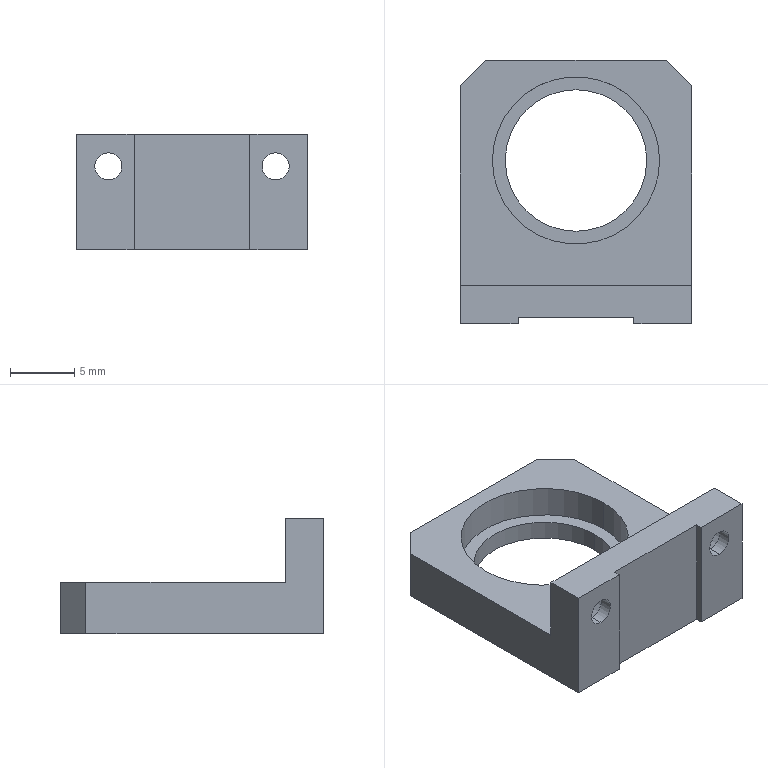Part | SolidWorks | features MoveFace 4, ICE 2, BaseBody 1, Chamfer 1, DelFace 1, HoleWzd 1 | 1 solid | 29 faces | box 18 x 20.5 x 9 mm | volume 1150 mm3 | plane 17 | cylinder 12 | commonest cylinder face diameters 2.1 x4 4.3 x4 11 x2 13 x2
STEP:
#1=CARTESIAN_POINT('',(6.,1.,7.6));
#2=VERTEX_POINT('',#1);
#3=CARTESIAN_POINT('',(6.,1.,11.9));
#4=VERTEX_POINT('',#3);
#5=CARTESIAN_POINT('',(6.,1.,9.75));
#6=DIRECTION('',(0.,1.,0.));
#7=DIRECTION('',(0.,0.,1.));
#8=AXIS2_PLACEMENT_3D('',#5,#6,#7);
#9=CIRCLE('',#8,2.15);
#10=EDGE_CURVE('',#2,#4,#9,.T.);
#11=ORIENTED_EDGE('',*,*,#10,.F.);
#12=CARTESIAN_POINT('',(6.,3.,7.6));
#13=VERTEX_POINT('',#12);
#14=CARTESIAN_POINT('',(6.,3.,7.6));
#15=DIRECTION('',(0.,1.,0.));
#16=VECTOR('',#15,1000.);
#17=LINE('',#14,#16);
#18=EDGE_CURVE('',#2,#13,#17,.T.);
#19=ORIENTED_EDGE('',*,*,#18,.T.);
#20=CARTESIAN_POINT('',(6.,3.,11.9));
#21=VERTEX_POINT('',#20);
#22=CARTESIAN_POINT('',(6.,3.,9.75));
#23=DIRECTION('',(0.,1.,0.));
#24=DIRECTION('',(0.,0.,1.));
#25=AXIS2_PLACEMENT_3D('',#22,#23,#24);
#26=CIRCLE('',#25,2.15);
#27=EDGE_CURVE('',#13,#21,#26,.T.);
#28=ORIENTED_EDGE('',*,*,#27,.T.);
#29=CARTESIAN_POINT('',(6.,3.,11.9));
#30=DIRECTION('',(0.,1.,0.));
#31=VECTOR('',#30,1000.);
#32=LINE('',#29,#31);
#33=EDGE_CURVE('',#4,#21,#32,.T.);
#34=ORIENTED_EDGE('',*,*,#33,.F.);
#35=EDGE_LOOP('',(#11,#19,#28,#34));
#36=FACE_OUTER_BOUND('',#35,.T.);
#37=CARTESIAN_POINT('',(6.,3.,9.75));
#38=DIRECTION('',(0.,1.,0.));
#39=DIRECTION('',(0.,0.,1.));
#40=AXIS2_PLACEMENT_3D('',#37,#38,#39);
#41=CYLINDRICAL_SURFACE('',#40,2.15);
#42=ADVANCED_FACE('',(#36),#41,.F.);
#43=CARTESIAN_POINT('',(6.,0.,10.8));
#44=VERTEX_POINT('',#43);
#45=CARTESIAN_POINT('',(6.,0.,8.7));
#46=VERTEX_POINT('',#45);
#47=CARTESIAN_POINT('',(6.,0.,9.75));
#48=DIRECTION('',(0.,-1.,0.));
#49=DIRECTION('',(0.,0.,-1.));
#50=AXIS2_PLACEMENT_3D('',#47,#48,#49);
#51=CIRCLE('',#50,1.05);
#52=EDGE_CURVE('',#44,#46,#51,.T.);
#53=ORIENTED_EDGE('',*,*,#52,.T.);
#54=CARTESIAN_POINT('',(6.,1.,8.7));
#55=VERTEX_POINT('',#54);
#56=CARTESIAN_POINT('',(6.,3.,8.7));
#57=DIRECTION('',(0.,1.,0.));
#58=VECTOR('',#57,1000.);
#59=LINE('',#56,#58);
#60=EDGE_CURVE('',#46,#55,#59,.T.);
#61=ORIENTED_EDGE('',*,*,#60,.T.);
#62=CARTESIAN_POINT('',(6.,1.,10.8));
#63=VERTEX_POINT('',#62);
#64=CARTESIAN_POINT('',(6.,1.,9.75));
#65=DIRECTION('',(0.,1.,0.));
#66=DIRECTION('',(0.,0.,1.));
#67=AXIS2_PLACEMENT_3D('',#64,#65,#66);
#68=CIRCLE('',#67,1.05);
#69=EDGE_CURVE('',#55,#63,#68,.T.);
#70=ORIENTED_EDGE('',*,*,#69,.T.);
#71=CARTESIAN_POINT('',(6.,3.,10.8));
#72=DIRECTION('',(0.,1.,0.));
#73=VECTOR('',#72,1000.);
#74=LINE('',#71,#73);
#75=EDGE_CURVE('',#44,#63,#74,.T.);
#76=ORIENTED_EDGE('',*,*,#75,.F.);
#77=EDGE_LOOP('',(#53,#61,#70,#76));
#78=FACE_OUTER_BOUND('',#77,.T.);
#79=CARTESIAN_POINT('',(6.,3.,9.75));
#80=DIRECTION('',(0.,1.,0.));
#81=DIRECTION('',(0.,0.,1.));
#82=AXIS2_PLACEMENT_3D('',#79,#80,#81);
#83=CYLINDRICAL_SURFACE('',#82,1.05);
#84=ADVANCED_FACE('',(#78),#83,.F.);
#85=CARTESIAN_POINT('',(19.,1.,7.6));
#86=VERTEX_POINT('',#85);
#87=CARTESIAN_POINT('',(19.,1.,11.9));
#88=VERTEX_POINT('',#87);
#89=CARTESIAN_POINT('',(19.,1.,9.75));
#90=DIRECTION('',(0.,1.,0.));
#91=DIRECTION('',(0.,0.,1.));
#92=AXIS2_PLACEMENT_3D('',#89,#90,#91);
#93=CIRCLE('',#92,2.15);
#94=EDGE_CURVE('',#86,#88,#93,.T.);
#95=ORIENTED_EDGE('',*,*,#94,.F.);
#96=CARTESIAN_POINT('',(19.,3.,7.6));
#97=VERTEX_POINT('',#96);
#98=CARTESIAN_POINT('',(19.,3.,7.6));
#99=DIRECTION('',(0.,1.,0.));
#100=VECTOR('',#99,1000.);
#101=LINE('',#98,#100);
#102=EDGE_CURVE('',#86,#97,#101,.T.);
#103=ORIENTED_EDGE('',*,*,#102,.T.);
#104=CARTESIAN_POINT('',(19.,3.,11.9));
#105=VERTEX_POINT('',#104);
#106=CARTESIAN_POINT('',(19.,3.,9.75));
#107=DIRECTION('',(0.,1.,0.));
#108=DIRECTION('',(0.,0.,1.));
#109=AXIS2_PLACEMENT_3D('',#106,#107,#108);
#110=CIRCLE('',#109,2.15);
#111=EDGE_CURVE('',#97,#105,#110,.T.);
#112=ORIENTED_EDGE('',*,*,#111,.T.);
#113=CARTESIAN_POINT('',(19.,3.,11.9));
#114=DIRECTION('',(0.,1.,0.));
#115=VECTOR('',#114,1000.);
#116=LINE('',#113,#115);
#117=EDGE_CURVE('',#88,#105,#116,.T.);
#118=ORIENTED_EDGE('',*,*,#117,.F.);
#119=EDGE_LOOP('',(#95,#103,#112,#118));
#120=FACE_OUTER_BOUND('',#119,.T.);
#121=CARTESIAN_POINT('',(19.,3.,9.75));
#122=DIRECTION('',(0.,1.,0.));
#123=DIRECTION('',(0.,0.,1.));
#124=AXIS2_PLACEMENT_3D('',#121,#122,#123);
#125=CYLINDRICAL_SURFACE('',#124,2.15);
#126=ADVANCED_FACE('',(#120),#125,.F.);
#127=CARTESIAN_POINT('',(19.,0.,10.8));
#128=VERTEX_POINT('',#127);
#129=CARTESIAN_POINT('',(19.,0.,8.7));
#130=VERTEX_POINT('',#129);
#131=CARTESIAN_POINT('',(19.,0.,9.75));
#132=DIRECTION('',(0.,-1.,0.));
#133=DIRECTION('',(0.,0.,-1.));
#134=AXIS2_PLACEMENT_3D('',#131,#132,#133);
#135=CIRCLE('',#134,1.05);
#136=EDGE_CURVE('',#128,#130,#135,.T.);
#137=ORIENTED_EDGE('',*,*,#136,.T.);
#138=CARTESIAN_POINT('',(19.,1.,8.7));
#139=VERTEX_POINT('',#138);
#140=CARTESIAN_POINT('',(19.,3.,8.7));
#141=DIRECTION('',(0.,1.,0.));
#142=VECTOR('',#141,1000.);
#143=LINE('',#140,#142);
#144=EDGE_CURVE('',#130,#139,#143,.T.);
#145=ORIENTED_EDGE('',*,*,#144,.T.);
#146=CARTESIAN_POINT('',(19.,1.,10.8));
#147=VERTEX_POINT('',#146);
#148=CARTESIAN_POINT('',(19.,1.,9.75));
#149=DIRECTION('',(0.,1.,0.));
#150=DIRECTION('',(0.,0.,1.));
#151=AXIS2_PLACEMENT_3D('',#148,#149,#150);
#152=CIRCLE('',#151,1.05);
#153=EDGE_CURVE('',#139,#147,#152,.T.);
#154=ORIENTED_EDGE('',*,*,#153,.T.);
#155=CARTESIAN_POINT('',(19.,3.,10.8));
#156=DIRECTION('',(0.,1.,0.));
#157=VECTOR('',#156,1000.);
#158=LINE('',#155,#157);
#159=EDGE_CURVE('',#128,#147,#158,.T.);
#160=ORIENTED_EDGE('',*,*,#159,.F.);
#161=EDGE_LOOP('',(#137,#145,#154,#160));
#162=FACE_OUTER_BOUND('',#161,.T.);
#163=CARTESIAN_POINT('',(19.,3.,9.75));
#164=DIRECTION('',(0.,1.,0.));
#165=DIRECTION('',(0.,0.,1.));
#166=AXIS2_PLACEMENT_3D('',#163,#164,#165);
#167=CYLINDRICAL_SURFACE('',#166,1.05);
#168=ADVANCED_FACE('',(#162),#167,.F.);
#169=CARTESIAN_POINT('',(18.,12.7,3.25));
#170=VERTEX_POINT('',#169);
#171=CARTESIAN_POINT('',(7.,12.7,3.25));
#172=VERTEX_POINT('',#171);
#173=CARTESIAN_POINT('',(12.5,12.7,3.25));
#174=DIRECTION('',(0.,0.,-1.));
#175=DIRECTION('',(1.,0.,0.));
#176=AXIS2_PLACEMENT_3D('',#173,#174,#175);
#177=CIRCLE('',#176,5.5);
#178=EDGE_CURVE('',#170,#172,#177,.T.);
#179=ORIENTED_EDGE('',*,*,#178,.T.);
#180=CARTESIAN_POINT('',(7.,12.7,4.75));
#181=VERTEX_POINT('',#180);
#182=CARTESIAN_POINT('',(7.,12.7,11.25));
#183=DIRECTION('',(0.,0.,1.));
#184=VECTOR('',#183,1000.);
#185=LINE('',#182,#184);
#186=EDGE_CURVE('',#172,#181,#185,.T.);
#187=ORIENTED_EDGE('',*,*,#186,.T.);
#188=CARTESIAN_POINT('',(18.,12.7,4.75));
#189=VERTEX_POINT('',#188);
#190=CARTESIAN_POINT('',(12.5,12.7,4.75));
#191=DIRECTION('',(0.,0.,-1.));
#192=DIRECTION('',(1.,0.,0.));
#193=AXIS2_PLACEMENT_3D('',#190,#191,#192);
#194=CIRCLE('',#193,5.5);
#195=EDGE_CURVE('',#189,#181,#194,.T.);
#196=ORIENTED_EDGE('',*,*,#195,.F.);
#197=CARTESIAN_POINT('',(18.,12.7,11.25));
#198=DIRECTION('',(0.,0.,1.));
#199=VECTOR('',#198,1000.);
#200=LINE('',#197,#199);
#201=EDGE_CURVE('',#170,#189,#200,.T.);
#202=ORIENTED_EDGE('',*,*,#201,.F.);
#203=EDGE_LOOP('',(#179,#187,#196,#202));
#204=FACE_OUTER_BOUND('',#203,.T.);
#205=CARTESIAN_POINT('',(12.5,12.7,11.25));
#206=DIRECTION('',(0.,0.,1.));
#207=DIRECTION('',(1.,0.,0.));
#208=AXIS2_PLACEMENT_3D('',#205,#206,#207);
#209=CYLINDRICAL_SURFACE('',#208,5.5);
#210=ADVANCED_FACE('',(#204),#209,.F.);
#211=CARTESIAN_POINT('',(19.,12.7,4.75));
#212=VERTEX_POINT('',#211);
#213=CARTESIAN_POINT('',(6.,12.7,4.75));
#214=VERTEX_POINT('',#213);
#215=CARTESIAN_POINT('',(12.5,12.7,4.75));
#216=DIRECTION('',(0.,0.,-1.));
#217=DIRECTION('',(1.,0.,0.));
#218=AXIS2_PLACEMENT_3D('',#215,#216,#217);
#219=CIRCLE('',#218,6.5);
#220=EDGE_CURVE('',#212,#214,#219,.T.);
#221=ORIENTED_EDGE('',*,*,#220,.T.);
#222=CARTESIAN_POINT('',(6.,12.7,7.25));
#223=VERTEX_POINT('',#222);
#224=CARTESIAN_POINT('',(6.,12.7,11.25));
#225=DIRECTION('',(0.,0.,1.));
#226=VECTOR('',#225,1000.);
#227=LINE('',#224,#226);
#228=EDGE_CURVE('',#214,#223,#227,.T.);
#229=ORIENTED_EDGE('',*,*,#228,.T.);
#230=CARTESIAN_POINT('',(19.,12.7,7.25));
#231=VERTEX_POINT('',#230);
#232=CARTESIAN_POINT('',(12.5,12.7,7.25));
#233=DIRECTION('',(0.,0.,1.));
#234=DIRECTION('',(-1.,0.,0.));
#235=AXIS2_PLACEMENT_3D('',#232,#233,#234);
#236=CIRCLE('',#235,6.5);
#237=EDGE_CURVE('',#223,#231,#236,.T.);
#238=ORIENTED_EDGE('',*,*,#237,.T.);
#239=CARTESIAN_POINT('',(19.,12.7,11.25));
#240=DIRECTION('',(0.,0.,1.));
#241=VECTOR('',#240,1000.);
#242=LINE('',#239,#241);
#243=EDGE_CURVE('',#212,#231,#242,.T.);
#244=ORIENTED_EDGE('',*,*,#243,.F.);
#245=EDGE_LOOP('',(#221,#229,#238,#244));
#246=FACE_OUTER_BOUND('',#245,.T.);
#247=CARTESIAN_POINT('',(12.5,12.7,11.25));
#248=DIRECTION('',(0.,0.,1.));
#249=DIRECTION('',(1.,0.,0.));
#250=AXIS2_PLACEMENT_3D('',#247,#248,#249);
#251=CYLINDRICAL_SURFACE('',#250,6.5);
#252=ADVANCED_FACE('',(#246),#251,.F.);
#253=CARTESIAN_POINT('',(3.5,3.,12.25));
#254=VERTEX_POINT('',#253);
#255=CARTESIAN_POINT('',(21.5,3.,12.25));
#256=VERTEX_POINT('',#255);
#257=CARTESIAN_POINT('',(0.,3.,12.25));
#258=DIRECTION('',(1.,0.,0.));
#259=VECTOR('',#258,1000.);
#260=LINE('',#257,#259);
#261=EDGE_CURVE('',#254,#256,#260,.T.);
#262=ORIENTED_EDGE('',*,*,#261,.F.);
#263=CARTESIAN_POINT('',(3.5,0.,12.25));
#264=VERTEX_POINT('',#263);
#265=CARTESIAN_POINT('',(3.5,0.,12.25));
#266=DIRECTION('',(0.,-1.,0.));
#267=VECTOR('',#266,1000.);
#268=LINE('',#265,#267);
#269=EDGE_CURVE('',#254,#264,#268,.T.);
#270=ORIENTED_EDGE('',*,*,#269,.T.);
#271=CARTESIAN_POINT('',(8.,0.,12.25));
#272=VERTEX_POINT('',#271);
#273=CARTESIAN_POINT('',(0.,0.,12.25));
#274=DIRECTION('',(-1.,0.,0.));
#275=VECTOR('',#274,1000.);
#276=LINE('',#273,#275);
#277=EDGE_CURVE('',#272,#264,#276,.T.);
#278=ORIENTED_EDGE('',*,*,#277,.F.);
#279=CARTESIAN_POINT('',(8.,0.5,12.25));
#280=VERTEX_POINT('',#279);
#281=CARTESIAN_POINT('',(8.,0.,12.25));
#282=DIRECTION('',(0.,1.,0.));
#283=VECTOR('',#282,1000.);
#284=LINE('',#281,#283);
#285=EDGE_CURVE('',#272,#280,#284,.T.);
#286=ORIENTED_EDGE('',*,*,#285,.T.);
#287=CARTESIAN_POINT('',(17.,0.5,12.25));
#288=VERTEX_POINT('',#287);
#289=CARTESIAN_POINT('',(6.,0.5,12.25));
#290=DIRECTION('',(1.,0.,0.));
#291=VECTOR('',#290,1000.);
#292=LINE('',#289,#291);
#293=EDGE_CURVE('',#280,#288,#292,.T.);
#294=ORIENTED_EDGE('',*,*,#293,.T.);
#295=CARTESIAN_POINT('',(17.,0.,12.25));
#296=VERTEX_POINT('',#295);
#297=CARTESIAN_POINT('',(17.,0.,12.25));
#298=DIRECTION('',(0.,-1.,0.));
#299=VECTOR('',#298,1000.);
#300=LINE('',#297,#299);
#301=EDGE_CURVE('',#288,#296,#300,.T.);
#302=ORIENTED_EDGE('',*,*,#301,.T.);
#303=CARTESIAN_POINT('',(21.5,0.,12.25));
#304=VERTEX_POINT('',#303);
#305=CARTESIAN_POINT('',(0.,0.,12.25));
#306=DIRECTION('',(-1.,0.,0.));
#307=VECTOR('',#306,1000.);
#308=LINE('',#305,#307);
#309=EDGE_CURVE('',#304,#296,#308,.T.);
#310=ORIENTED_EDGE('',*,*,#309,.F.);
#311=CARTESIAN_POINT('',(21.5,0.,12.25));
#312=DIRECTION('',(0.,1.,0.));
#313=VECTOR('',#312,1000.);
#314=LINE('',#311,#313);
#315=EDGE_CURVE('',#304,#256,#314,.T.);
#316=ORIENTED_EDGE('',*,*,#315,.T.);
#317=EDGE_LOOP('',(#262,#270,#278,#286,#294,#302,#310,#316));
#318=FACE_OUTER_BOUND('',#317,.T.);
#319=CARTESIAN_POINT('',(0.,0.,12.25));
#320=DIRECTION('',(0.,0.,1.));
#321=DIRECTION('',(1.,0.,0.));
#322=AXIS2_PLACEMENT_3D('',#319,#320,#321);
#323=PLANE('',#322);
#324=ADVANCED_FACE('',(#318),#323,.T.);
#325=ORIENTED_EDGE('',*,*,#52,.F.);
#326=CARTESIAN_POINT('',(6.,0.,9.75));
#327=DIRECTION('',(0.,-1.,0.));
#328=DIRECTION('',(0.,0.,-1.));
#329=AXIS2_PLACEMENT_3D('',#326,#327,#328);
#330=CIRCLE('',#329,1.05);
#331=EDGE_CURVE('',#46,#44,#330,.T.);
#332=ORIENTED_EDGE('',*,*,#331,.F.);
#333=EDGE_LOOP('',(#325,#332));
#334=FACE_BOUND('',#333,.T.);
#335=ORIENTED_EDGE('',*,*,#277,.T.);
#336=CARTESIAN_POINT('',(3.5,0.,3.25));
#337=VERTEX_POINT('',#336);
#338=CARTESIAN_POINT('',(3.5,0.,19.25));
#339=DIRECTION('',(0.,0.,-1.));
#340=VECTOR('',#339,1000.);
#341=LINE('',#338,#340);
#342=EDGE_CURVE('',#264,#337,#341,.T.);
#343=ORIENTED_EDGE('',*,*,#342,.T.);
#344=CARTESIAN_POINT('',(8.,0.,3.25));
#345=VERTEX_POINT('',#344);
#346=CARTESIAN_POINT('',(0.,0.,3.25));
#347=DIRECTION('',(1.,0.,0.));
#348=VECTOR('',#347,1000.);
#349=LINE('',#346,#348);
#350=EDGE_CURVE('',#337,#345,#349,.T.);
#351=ORIENTED_EDGE('',*,*,#350,.T.);
#352=CARTESIAN_POINT('',(8.,0.,3.25));
#353=DIRECTION('',(0.,0.,1.));
#354=VECTOR('',#353,1000.);
#355=LINE('',#352,#354);
#356=EDGE_CURVE('',#345,#272,#355,.T.);
#357=ORIENTED_EDGE('',*,*,#356,.T.);
#358=EDGE_LOOP('',(#335,#343,#351,#357));
#359=FACE_OUTER_BOUND('',#358,.T.);
#360=CARTESIAN_POINT('',(0.,0.,3.25));
#361=DIRECTION('',(0.,-1.,0.));
#362=DIRECTION('',(0.,0.,-1.));
#363=AXIS2_PLACEMENT_3D('',#360,#361,#362);
#364=PLANE('',#363);
#365=ADVANCED_FACE('',(#334,#359),#364,.T.);
#366=ORIENTED_EDGE('',*,*,#136,.F.);
#367=CARTESIAN_POINT('',(19.,0.,9.75));
#368=DIRECTION('',(0.,-1.,0.));
#369=DIRECTION('',(0.,0.,-1.));
#370=AXIS2_PLACEMENT_3D('',#367,#368,#369);
#371=CIRCLE('',#370,1.05);
#372=EDGE_CURVE('',#130,#128,#371,.T.);
#373=ORIENTED_EDGE('',*,*,#372,.F.);
#374=EDGE_LOOP('',(#366,#373));
#375=FACE_BOUND('',#374,.T.);
#376=CARTESIAN_POINT('',(17.,0.,3.25));
#377=VERTEX_POINT('',#376);
#378=CARTESIAN_POINT('',(21.5,0.,3.25));
#379=VERTEX_POINT('',#378);
#380=CARTESIAN_POINT('',(0.,0.,3.25));
#381=DIRECTION('',(1.,0.,0.));
#382=VECTOR('',#381,1000.);
#383=LINE('',#380,#382);
#384=EDGE_CURVE('',#377,#379,#383,.T.);
#385=ORIENTED_EDGE('',*,*,#384,.T.);
#386=CARTESIAN_POINT('',(21.5,0.,19.25));
#387=DIRECTION('',(0.,0.,-1.));
#388=VECTOR('',#387,1000.);
#389=LINE('',#386,#388);
#390=EDGE_CURVE('',#304,#379,#389,.T.);
#391=ORIENTED_EDGE('',*,*,#390,.F.);
#392=ORIENTED_EDGE('',*,*,#309,.T.);
#393=CARTESIAN_POINT('',(17.,0.,3.25));
#394=DIRECTION('',(0.,0.,-1.));
#395=VECTOR('',#394,1000.);
#396=LINE('',#393,#395);
#397=EDGE_CURVE('',#296,#377,#396,.T.);
#398=ORIENTED_EDGE('',*,*,#397,.T.);
#399=EDGE_LOOP('',(#385,#391,#392,#398));
#400=FACE_OUTER_BOUND('',#399,.T.);
#401=CARTESIAN_POINT('',(0.,0.,3.25));
#402=DIRECTION('',(0.,-1.,0.));
#403=DIRECTION('',(0.,0.,-1.));
#404=AXIS2_PLACEMENT_3D('',#401,#402,#403);
#405=PLANE('',#404);
#406=ADVANCED_FACE('',(#375,#400),#405,.T.);
#407=CARTESIAN_POINT('',(19.5,20.5,7.25));
#408=VERTEX_POINT('',#407);
#409=CARTESIAN_POINT('',(5.5,20.5,7.25));
#410=VERTEX_POINT('',#409);
#411=CARTESIAN_POINT('',(25.,20.5,7.25));
#412=DIRECTION('',(-1.,0.,0.));
#413=VECTOR('',#412,1000.);
#414=LINE('',#411,#413);
#415=EDGE_CURVE('',#408,#410,#414,.T.);
#416=ORIENTED_EDGE('',*,*,#415,.F.);
#417=CARTESIAN_POINT('',(19.5,20.5,3.25));
#418=VERTEX_POINT('',#417);
#419=CARTESIAN_POINT('',(19.5,20.5,3.25));
#420=DIRECTION('',(0.,0.,-1.));
#421=VECTOR('',#420,1000.);
#422=LINE('',#419,#421);
#423=EDGE_CURVE('',#408,#418,#422,.T.);
#424=ORIENTED_EDGE('',*,*,#423,.T.);
#425=CARTESIAN_POINT('',(5.5,20.5,3.25));
#426=VERTEX_POINT('',#425);
#427=CARTESIAN_POINT('',(0.,20.5,3.25));
#428=DIRECTION('',(-1.,0.,0.));
#429=VECTOR('',#428,1000.);
#430=LINE('',#427,#429);
#431=EDGE_CURVE('',#418,#426,#430,.T.);
#432=ORIENTED_EDGE('',*,*,#431,.T.);
#433=CARTESIAN_POINT('',(5.5,20.5,3.25));
#434=DIRECTION('',(0.,0.,1.));
#435=VECTOR('',#434,1000.);
#436=LINE('',#433,#435);
#437=EDGE_CURVE('',#426,#410,#436,.T.);
#438=ORIENTED_EDGE('',*,*,#437,.T.);
#439=EDGE_LOOP('',(#416,#424,#432,#438));
#440=FACE_OUTER_BOUND('',#439,.T.);
#441=CARTESIAN_POINT('',(25.,20.5,3.25));
#442=DIRECTION('',(0.,1.,0.));
#443=DIRECTION('',(0.,0.,1.));
#444=AXIS2_PLACEMENT_3D('',#441,#442,#443);
#445=PLANE('',#444);
#446=ADVANCED_FACE('',(#440),#445,.T.);
#447=ORIENTED_EDGE('',*,*,#178,.F.);
#448=CARTESIAN_POINT('',(12.5,12.7,3.25));
#449=DIRECTION('',(0.,0.,-1.));
#450=DIRECTION('',(1.,0.,0.));
#451=AXIS2_PLACEMENT_3D('',#448,#449,#450);
#452=CIRCLE('',#451,5.5);
#453=EDGE_CURVE('',#172,#170,#452,.T.);
#454=ORIENTED_EDGE('',*,*,#453,.F.);
#455=EDGE_LOOP('',(#447,#454));
#456=FACE_BOUND('',#455,.T.);
#457=ORIENTED_EDGE('',*,*,#431,.F.);
#458=CARTESIAN_POINT('',(21.5,18.5,3.25));
#459=VERTEX_POINT('',#458);
#460=CARTESIAN_POINT('',(19.5,20.5,3.25));
#461=DIRECTION('',(0.7071,-0.7071,0.));
#462=VECTOR('',#461,1000.);
#463=LINE('',#460,#462);
#464=EDGE_CURVE('',#418,#459,#463,.T.);
#465=ORIENTED_EDGE('',*,*,#464,.T.);
#466=CARTESIAN_POINT('',(21.5,20.5,3.25));
#467=DIRECTION('',(0.,-1.,0.));
#468=VECTOR('',#467,1000.);
#469=LINE('',#466,#468);
#470=EDGE_CURVE('',#459,#379,#469,.T.);
#471=ORIENTED_EDGE('',*,*,#470,.T.);
#472=ORIENTED_EDGE('',*,*,#384,.F.);
#473=CARTESIAN_POINT('',(17.,0.5,3.25));
#474=VERTEX_POINT('',#473);
#475=CARTESIAN_POINT('',(17.,0.5,3.25));
#476=DIRECTION('',(0.,1.,0.));
#477=VECTOR('',#476,1000.);
#478=LINE('',#475,#477);
#479=EDGE_CURVE('',#377,#474,#478,.T.);
#480=ORIENTED_EDGE('',*,*,#479,.T.);
#481=CARTESIAN_POINT('',(8.,0.5,3.25));
#482=VERTEX_POINT('',#481);
#483=CARTESIAN_POINT('',(0.,0.5,3.25));
#484=DIRECTION('',(1.,0.,0.));
#485=VECTOR('',#484,1000.);
#486=LINE('',#483,#485);
#487=EDGE_CURVE('',#482,#474,#486,.T.);
#488=ORIENTED_EDGE('',*,*,#487,.F.);
#489=CARTESIAN_POINT('',(8.,0.,3.25));
#490=DIRECTION('',(0.,-1.,0.));
#491=VECTOR('',#490,1000.);
#492=LINE('',#489,#491);
#493=EDGE_CURVE('',#482,#345,#492,.T.);
#494=ORIENTED_EDGE('',*,*,#493,.T.);
#495=ORIENTED_EDGE('',*,*,#350,.F.);
#496=CARTESIAN_POINT('',(3.5,18.5,3.25));
#497=VERTEX_POINT('',#496);
#498=CARTESIAN_POINT('',(3.5,0.,3.25));
#499=DIRECTION('',(0.,1.,0.));
#500=VECTOR('',#499,1000.);
#501=LINE('',#498,#500);
#502=EDGE_CURVE('',#337,#497,#501,.T.);
#503=ORIENTED_EDGE('',*,*,#502,.T.);
#504=CARTESIAN_POINT('',(3.5,18.5,3.25));
#505=DIRECTION('',(0.7071,0.7071,0.));
#506=VECTOR('',#505,1000.);
#507=LINE('',#504,#506);
#508=EDGE_CURVE('',#497,#426,#507,.T.);
#509=ORIENTED_EDGE('',*,*,#508,.T.);
#510=EDGE_LOOP('',(#457,#465,#471,#472,#480,#488,#494,#495,#503,#509));
#511=FACE_OUTER_BOUND('',#510,.T.);
#512=CARTESIAN_POINT('',(0.,0.,3.25));
#513=DIRECTION('',(0.,0.,1.));
#514=DIRECTION('',(1.,0.,0.));
#515=AXIS2_PLACEMENT_3D('',#512,#513,#514);
#516=PLANE('',#515);
#517=ADVANCED_FACE('',(#456,#511),#516,.F.);
#518=CARTESIAN_POINT('',(12.5,12.7,7.25));
#519=DIRECTION('',(0.,0.,1.));
#520=DIRECTION('',(-1.,0.,0.));
#521=AXIS2_PLACEMENT_3D('',#518,#519,#520);
#522=CIRCLE('',#521,6.5);
#523=EDGE_CURVE('',#231,#223,#522,.T.);
#524=ORIENTED_EDGE('',*,*,#523,.F.);
#525=ORIENTED_EDGE('',*,*,#237,.F.);
#526=EDGE_LOOP('',(#524,#525));
#527=FACE_BOUND('',#526,.T.);
#528=CARTESIAN_POINT('',(21.5,18.5,7.25));
#529=VERTEX_POINT('',#528);
#530=CARTESIAN_POINT('',(21.5,3.,7.25));
#531=VERTEX_POINT('',#530);
#532=CARTESIAN_POINT('',(21.5,3.,7.25));
#533=DIRECTION('',(0.,-1.,0.));
#534=VECTOR('',#533,1000.);
#535=LINE('',#532,#534);
#536=EDGE_CURVE('',#529,#531,#535,.T.);
#537=ORIENTED_EDGE('',*,*,#536,.F.);
#538=CARTESIAN_POINT('',(19.5,20.5,7.25));
#539=DIRECTION('',(-0.7071,0.7071,0.));
#540=VECTOR('',#539,1000.);
#541=LINE('',#538,#540);
#542=EDGE_CURVE('',#529,#408,#541,.T.);
#543=ORIENTED_EDGE('',*,*,#542,.T.);
#544=ORIENTED_EDGE('',*,*,#415,.T.);
#545=CARTESIAN_POINT('',(3.5,18.5,7.25));
#546=VERTEX_POINT('',#545);
#547=CARTESIAN_POINT('',(3.5,18.5,7.25));
#548=DIRECTION('',(-0.7071,-0.7071,0.));
#549=VECTOR('',#548,1000.);
#550=LINE('',#547,#549);
#551=EDGE_CURVE('',#410,#546,#550,.T.);
#552=ORIENTED_EDGE('',*,*,#551,.T.);
#553=CARTESIAN_POINT('',(3.5,3.,7.25));
#554=VERTEX_POINT('',#553);
#555=CARTESIAN_POINT('',(3.5,3.,7.25));
#556=DIRECTION('',(0.,1.,0.));
#557=VECTOR('',#556,1000.);
#558=LINE('',#555,#557);
#559=EDGE_CURVE('',#554,#546,#558,.T.);
#560=ORIENTED_EDGE('',*,*,#559,.F.);
#561=CARTESIAN_POINT('',(25.,3.,7.25));
#562=DIRECTION('',(-1.,0.,0.));
#563=VECTOR('',#562,1000.);
#564=LINE('',#561,#563);
#565=EDGE_CURVE('',#531,#554,#564,.T.);
#566=ORIENTED_EDGE('',*,*,#565,.F.);
#567=EDGE_LOOP('',(#537,#543,#544,#552,#560,#566));
#568=FACE_OUTER_BOUND('',#567,.T.);
#569=CARTESIAN_POINT('',(25.,3.,7.25));
#570=DIRECTION('',(0.,0.,-1.));
#571=DIRECTION('',(-1.,0.,0.));
#572=AXIS2_PLACEMENT_3D('',#569,#570,#571);
#573=PLANE('',#572);
#574=ADVANCED_FACE('',(#527,#568),#573,.F.);
#575=CARTESIAN_POINT('',(6.,3.,9.75));
#576=DIRECTION('',(0.,1.,0.));
#577=DIRECTION('',(0.,0.,1.));
#578=AXIS2_PLACEMENT_3D('',#575,#576,#577);
#579=CIRCLE('',#578,2.15);
#580=EDGE_CURVE('',#21,#13,#579,.T.);
#581=ORIENTED_EDGE('',*,*,#580,.F.);
#582=ORIENTED_EDGE('',*,*,#27,.F.);
#583=EDGE_LOOP('',(#581,#582));
#584=FACE_BOUND('',#583,.T.);
#585=CARTESIAN_POINT('',(19.,3.,9.75));
#586=DIRECTION('',(0.,1.,0.));
#587=DIRECTION('',(0.,0.,1.));
#588=AXIS2_PLACEMENT_3D('',#585,#586,#587);
#589=CIRCLE('',#588,2.15);
#590=EDGE_CURVE('',#105,#97,#589,.T.);
#591=ORIENTED_EDGE('',*,*,#590,.F.);
#592=ORIENTED_EDGE('',*,*,#111,.F.);
#593=EDGE_LOOP('',(#591,#592));
#594=FACE_BOUND('',#593,.T.);
#595=ORIENTED_EDGE('',*,*,#565,.T.);
#596=CARTESIAN_POINT('',(3.5,3.,0.));
#597=DIRECTION('',(0.,0.,1.));
#598=VECTOR('',#597,1000.);
#599=LINE('',#596,#598);
#600=EDGE_CURVE('',#554,#254,#599,.T.);
#601=ORIENTED_EDGE('',*,*,#600,.T.);
#602=ORIENTED_EDGE('',*,*,#261,.T.);
#603=CARTESIAN_POINT('',(21.5,3.,0.));
#604=DIRECTION('',(0.,0.,-1.));
#605=VECTOR('',#604,1000.);
#606=LINE('',#603,#605);
#607=EDGE_CURVE('',#256,#531,#606,.T.);
#608=ORIENTED_EDGE('',*,*,#607,.T.);
#609=EDGE_LOOP('',(#595,#601,#602,#608));
#610=FACE_OUTER_BOUND('',#609,.T.);
#611=CARTESIAN_POINT('',(0.,3.,0.));
#612=DIRECTION('',(0.,1.,0.));
#613=DIRECTION('',(0.,0.,1.));
#614=AXIS2_PLACEMENT_3D('',#611,#612,#613);
#615=PLANE('',#614);
#616=ADVANCED_FACE('',(#584,#594,#610),#615,.T.);
#617=ORIENTED_EDGE('',*,*,#186,.F.);
#618=ORIENTED_EDGE('',*,*,#453,.T.);
#619=ORIENTED_EDGE('',*,*,#201,.T.);
#620=CARTESIAN_POINT('',(12.5,12.7,4.75));
#621=DIRECTION('',(0.,0.,-1.));
#622=DIRECTION('',(1.,0.,0.));
#623=AXIS2_PLACEMENT_3D('',#620,#621,#622);
#624=CIRCLE('',#623,5.5);
#625=EDGE_CURVE('',#181,#189,#624,.T.);
#626=ORIENTED_EDGE('',*,*,#625,.F.);
#627=EDGE_LOOP('',(#617,#618,#619,#626));
#628=FACE_OUTER_BOUND('',#627,.T.);
#629=CARTESIAN_POINT('',(12.5,12.7,11.25));
#630=DIRECTION('',(0.,0.,1.));
#631=DIRECTION('',(1.,0.,0.));
#632=AXIS2_PLACEMENT_3D('',#629,#630,#631);
#633=CYLINDRICAL_SURFACE('',#632,5.5);
#634=ADVANCED_FACE('',(#628),#633,.F.);
#635=ORIENTED_EDGE('',*,*,#293,.F.);
#636=CARTESIAN_POINT('',(8.,0.5,11.25));
#637=DIRECTION('',(0.,0.,1.));
#638=VECTOR('',#637,1000.);
#639=LINE('',#636,#638);
#640=EDGE_CURVE('',#482,#280,#639,.T.);
#641=ORIENTED_EDGE('',*,*,#640,.F.);
#642=ORIENTED_EDGE('',*,*,#487,.T.);
#643=CARTESIAN_POINT('',(17.,0.5,11.25));
#644=DIRECTION('',(0.,0.,-1.));
#645=VECTOR('',#644,1000.);
#646=LINE('',#643,#645);
#647=EDGE_CURVE('',#288,#474,#646,.T.);
#648=ORIENTED_EDGE('',*,*,#647,.F.);
#649=EDGE_LOOP('',(#635,#641,#642,#648));
#650=FACE_OUTER_BOUND('',#649,.T.);
#651=CARTESIAN_POINT('',(6.,0.5,11.25));
#652=DIRECTION('',(0.,1.,0.));
#653=DIRECTION('',(0.,0.,1.));
#654=AXIS2_PLACEMENT_3D('',#651,#652,#653);
#655=PLANE('',#654);
#656=ADVANCED_FACE('',(#650),#655,.F.);
#657=ORIENTED_EDGE('',*,*,#195,.T.);
#658=ORIENTED_EDGE('',*,*,#625,.T.);
#659=EDGE_LOOP('',(#657,#658));
#660=FACE_BOUND('',#659,.T.);
#661=ORIENTED_EDGE('',*,*,#220,.F.);
#662=CARTESIAN_POINT('',(12.5,12.7,4.75));
#663=DIRECTION('',(0.,0.,-1.));
#664=DIRECTION('',(1.,0.,0.));
#665=AXIS2_PLACEMENT_3D('',#662,#663,#664);
#666=CIRCLE('',#665,6.5);
#667=EDGE_CURVE('',#214,#212,#666,.T.);
#668=ORIENTED_EDGE('',*,*,#667,.F.);
#669=EDGE_LOOP('',(#661,#668));
#670=FACE_OUTER_BOUND('',#669,.T.);
#671=CARTESIAN_POINT('',(18.,12.7,4.75));
#672=DIRECTION('',(0.,0.,-1.));
#673=DIRECTION('',(-1.,0.,0.));
#674=AXIS2_PLACEMENT_3D('',#671,#672,#673);
#675=PLANE('',#674);
#676=ADVANCED_FACE('',(#660,#670),#675,.F.);
#677=ORIENTED_EDGE('',*,*,#301,.F.);
#678=ORIENTED_EDGE('',*,*,#647,.T.);
#679=ORIENTED_EDGE('',*,*,#479,.F.);
#680=ORIENTED_EDGE('',*,*,#397,.F.);
#681=EDGE_LOOP('',(#677,#678,#679,#680));
#682=FACE_OUTER_BOUND('',#681,.T.);
#683=CARTESIAN_POINT('',(17.,0.5,11.25));
#684=DIRECTION('',(1.,0.,0.));
#685=DIRECTION('',(0.,0.,-1.));
#686=AXIS2_PLACEMENT_3D('',#683,#684,#685);
#687=PLANE('',#686);
#688=ADVANCED_FACE('',(#682),#687,.F.);
#689=ORIENTED_EDGE('',*,*,#285,.F.);
#690=ORIENTED_EDGE('',*,*,#356,.F.);
#691=ORIENTED_EDGE('',*,*,#493,.F.);
#692=ORIENTED_EDGE('',*,*,#640,.T.);
#693=EDGE_LOOP('',(#689,#690,#691,#692));
#694=FACE_OUTER_BOUND('',#693,.T.);
#695=CARTESIAN_POINT('',(8.,0.,11.25));
#696=DIRECTION('',(-1.,0.,0.));
#697=DIRECTION('',(0.,-1.,0.));
#698=AXIS2_PLACEMENT_3D('',#695,#696,#697);
#699=PLANE('',#698);
#700=ADVANCED_FACE('',(#694),#699,.F.);
#701=ORIENTED_EDGE('',*,*,#228,.F.);
#702=ORIENTED_EDGE('',*,*,#667,.T.);
#703=ORIENTED_EDGE('',*,*,#243,.T.);
#704=ORIENTED_EDGE('',*,*,#523,.T.);
#705=EDGE_LOOP('',(#701,#702,#703,#704));
#706=FACE_OUTER_BOUND('',#705,.T.);
#707=CARTESIAN_POINT('',(12.5,12.7,11.25));
#708=DIRECTION('',(0.,0.,1.));
#709=DIRECTION('',(1.,0.,0.));
#710=AXIS2_PLACEMENT_3D('',#707,#708,#709);
#711=CYLINDRICAL_SURFACE('',#710,6.5);
#712=ADVANCED_FACE('',(#706),#711,.F.);
#713=ORIENTED_EDGE('',*,*,#470,.F.);
#714=CARTESIAN_POINT('',(21.5,18.5,19.25));
#715=DIRECTION('',(0.,0.,1.));
#716=VECTOR('',#715,1000.);
#717=LINE('',#714,#716);
#718=EDGE_CURVE('',#459,#529,#717,.T.);
#719=ORIENTED_EDGE('',*,*,#718,.T.);
#720=ORIENTED_EDGE('',*,*,#536,.T.);
#721=ORIENTED_EDGE('',*,*,#607,.F.);
#722=ORIENTED_EDGE('',*,*,#315,.F.);
#723=ORIENTED_EDGE('',*,*,#390,.T.);
#724=EDGE_LOOP('',(#713,#719,#720,#721,#722,#723));
#725=FACE_OUTER_BOUND('',#724,.T.);
#726=CARTESIAN_POINT('',(21.5,20.5,19.25));
#727=DIRECTION('',(1.,0.,0.));
#728=DIRECTION('',(0.,1.,0.));
#729=AXIS2_PLACEMENT_3D('',#726,#727,#728);
#730=PLANE('',#729);
#731=ADVANCED_FACE('',(#725),#730,.T.);
#732=ORIENTED_EDGE('',*,*,#559,.T.);
#733=CARTESIAN_POINT('',(3.5,18.5,19.25));
#734=DIRECTION('',(0.,0.,-1.));
#735=VECTOR('',#734,1000.);
#736=LINE('',#733,#735);
#737=EDGE_CURVE('',#546,#497,#736,.T.);
#738=ORIENTED_EDGE('',*,*,#737,.T.);
#739=ORIENTED_EDGE('',*,*,#502,.F.);
#740=ORIENTED_EDGE('',*,*,#342,.F.);
#741=ORIENTED_EDGE('',*,*,#269,.F.);
#742=ORIENTED_EDGE('',*,*,#600,.F.);
#743=EDGE_LOOP('',(#732,#738,#739,#740,#741,#742));
#744=FACE_OUTER_BOUND('',#743,.T.);
#745=CARTESIAN_POINT('',(3.5,0.,19.25));
#746=DIRECTION('',(-1.,0.,0.));
#747=DIRECTION('',(0.,0.,1.));
#748=AXIS2_PLACEMENT_3D('',#745,#746,#747);
#749=PLANE('',#748);
#750=ADVANCED_FACE('',(#744),#749,.T.);
#751=ORIENTED_EDGE('',*,*,#542,.F.);
#752=ORIENTED_EDGE('',*,*,#718,.F.);
#753=ORIENTED_EDGE('',*,*,#464,.F.);
#754=ORIENTED_EDGE('',*,*,#423,.F.);
#755=EDGE_LOOP('',(#751,#752,#753,#754));
#756=FACE_OUTER_BOUND('',#755,.T.);
#757=CARTESIAN_POINT('',(19.5,20.5,3.25));
#758=DIRECTION('',(-0.7071,-0.7071,0.));
#759=DIRECTION('',(0.,0.,-1.));
#760=AXIS2_PLACEMENT_3D('',#757,#758,#759);
#761=PLANE('',#760);
#762=ADVANCED_FACE('',(#756),#761,.F.);
#763=ORIENTED_EDGE('',*,*,#551,.F.);
#764=ORIENTED_EDGE('',*,*,#437,.F.);
#765=ORIENTED_EDGE('',*,*,#508,.F.);
#766=ORIENTED_EDGE('',*,*,#737,.F.);
#767=EDGE_LOOP('',(#763,#764,#765,#766));
#768=FACE_OUTER_BOUND('',#767,.T.);
#769=CARTESIAN_POINT('',(3.5,18.5,19.25));
#770=DIRECTION('',(0.7071,-0.7071,0.));
#771=DIRECTION('',(0.,0.,-1.));
#772=AXIS2_PLACEMENT_3D('',#769,#770,#771);
#773=PLANE('',#772);
#774=ADVANCED_FACE('',(#768),#773,.F.);
#775=ORIENTED_EDGE('',*,*,#144,.F.);
#776=ORIENTED_EDGE('',*,*,#372,.T.);
#777=ORIENTED_EDGE('',*,*,#159,.T.);
#778=CARTESIAN_POINT('',(19.,1.,9.75));
#779=DIRECTION('',(0.,1.,0.));
#780=DIRECTION('',(0.,0.,1.));
#781=AXIS2_PLACEMENT_3D('',#778,#779,#780);
#782=CIRCLE('',#781,1.05);
#783=EDGE_CURVE('',#147,#139,#782,.T.);
#784=ORIENTED_EDGE('',*,*,#783,.T.);
#785=EDGE_LOOP('',(#775,#776,#777,#784));
#786=FACE_OUTER_BOUND('',#785,.T.);
#787=CARTESIAN_POINT('',(19.,3.,9.75));
#788=DIRECTION('',(0.,1.,0.));
#789=DIRECTION('',(0.,0.,1.));
#790=AXIS2_PLACEMENT_3D('',#787,#788,#789);
#791=CYLINDRICAL_SURFACE('',#790,1.05);
#792=ADVANCED_FACE('',(#786),#791,.F.);
#793=ORIENTED_EDGE('',*,*,#783,.F.);
#794=ORIENTED_EDGE('',*,*,#153,.F.);
#795=EDGE_LOOP('',(#793,#794));
#796=FACE_BOUND('',#795,.T.);
#797=CARTESIAN_POINT('',(19.,1.,9.75));
#798=DIRECTION('',(0.,1.,0.));
#799=DIRECTION('',(0.,0.,1.));
#800=AXIS2_PLACEMENT_3D('',#797,#798,#799);
#801=CIRCLE('',#800,2.15);
#802=EDGE_CURVE('',#88,#86,#801,.T.);
#803=ORIENTED_EDGE('',*,*,#802,.T.);
#804=ORIENTED_EDGE('',*,*,#94,.T.);
#805=EDGE_LOOP('',(#803,#804));
#806=FACE_OUTER_BOUND('',#805,.T.);
#807=CARTESIAN_POINT('',(20.05,1.,9.75));
#808=DIRECTION('',(0.,-1.,0.));
#809=DIRECTION('',(0.,0.,-1.));
#810=AXIS2_PLACEMENT_3D('',#807,#808,#809);
#811=PLANE('',#810);
#812=ADVANCED_FACE('',(#796,#806),#811,.F.);
#813=ORIENTED_EDGE('',*,*,#102,.F.);
#814=ORIENTED_EDGE('',*,*,#802,.F.);
#815=ORIENTED_EDGE('',*,*,#117,.T.);
#816=ORIENTED_EDGE('',*,*,#590,.T.);
#817=EDGE_LOOP('',(#813,#814,#815,#816));
#818=FACE_OUTER_BOUND('',#817,.T.);
#819=CARTESIAN_POINT('',(19.,3.,9.75));
#820=DIRECTION('',(0.,1.,0.));
#821=DIRECTION('',(0.,0.,1.));
#822=AXIS2_PLACEMENT_3D('',#819,#820,#821);
#823=CYLINDRICAL_SURFACE('',#822,2.15);
#824=ADVANCED_FACE('',(#818),#823,.F.);
#825=ORIENTED_EDGE('',*,*,#60,.F.);
#826=ORIENTED_EDGE('',*,*,#331,.T.);
#827=ORIENTED_EDGE('',*,*,#75,.T.);
#828=CARTESIAN_POINT('',(6.,1.,9.75));
#829=DIRECTION('',(0.,1.,0.));
#830=DIRECTION('',(0.,0.,1.));
#831=AXIS2_PLACEMENT_3D('',#828,#829,#830);
#832=CIRCLE('',#831,1.05);
#833=EDGE_CURVE('',#63,#55,#832,.T.);
#834=ORIENTED_EDGE('',*,*,#833,.T.);
#835=EDGE_LOOP('',(#825,#826,#827,#834));
#836=FACE_OUTER_BOUND('',#835,.T.);
#837=CARTESIAN_POINT('',(6.,3.,9.75));
#838=DIRECTION('',(0.,1.,0.));
#839=DIRECTION('',(0.,0.,1.));
#840=AXIS2_PLACEMENT_3D('',#837,#838,#839);
#841=CYLINDRICAL_SURFACE('',#840,1.05);
#842=ADVANCED_FACE('',(#836),#841,.F.);
#843=ORIENTED_EDGE('',*,*,#833,.F.);
#844=ORIENTED_EDGE('',*,*,#69,.F.);
#845=EDGE_LOOP('',(#843,#844));
#846=FACE_BOUND('',#845,.T.);
#847=CARTESIAN_POINT('',(6.,1.,9.75));
#848=DIRECTION('',(0.,1.,0.));
#849=DIRECTION('',(0.,0.,1.));
#850=AXIS2_PLACEMENT_3D('',#847,#848,#849);
#851=CIRCLE('',#850,2.15);
#852=EDGE_CURVE('',#4,#2,#851,.T.);
#853=ORIENTED_EDGE('',*,*,#852,.T.);
#854=ORIENTED_EDGE('',*,*,#10,.T.);
#855=EDGE_LOOP('',(#853,#854));
#856=FACE_OUTER_BOUND('',#855,.T.);
#857=CARTESIAN_POINT('',(7.05,1.,9.75));
#858=DIRECTION('',(0.,-1.,0.));
#859=DIRECTION('',(0.,0.,-1.));
#860=AXIS2_PLACEMENT_3D('',#857,#858,#859);
#861=PLANE('',#860);
#862=ADVANCED_FACE('',(#846,#856),#861,.F.);
#863=ORIENTED_EDGE('',*,*,#18,.F.);
#864=ORIENTED_EDGE('',*,*,#852,.F.);
#865=ORIENTED_EDGE('',*,*,#33,.T.);
#866=ORIENTED_EDGE('',*,*,#580,.T.);
#867=EDGE_LOOP('',(#863,#864,#865,#866));
#868=FACE_OUTER_BOUND('',#867,.T.);
#869=CARTESIAN_POINT('',(6.,3.,9.75));
#870=DIRECTION('',(0.,1.,0.));
#871=DIRECTION('',(0.,0.,1.));
#872=AXIS2_PLACEMENT_3D('',#869,#870,#871);
#873=CYLINDRICAL_SURFACE('',#872,2.15);
#874=ADVANCED_FACE('',(#868),#873,.F.);
#875=CLOSED_SHELL('',(#42,#84,#126,#168,#210,#252,#324,#365,#406,#446,#517,#574,#616,#634,#656,#676,#688,#700,#712,#731,#750,#762,#774,#792,#812,#824,#842,#862,#874));
#876=MANIFOLD_SOLID_BREP('',#875);
#877=CARTESIAN_POINT('',(0.,0.,0.));
#878=DIRECTION('',(0.,0.,1.));
#879=DIRECTION('',(1.,0.,0.));
#880=AXIS2_PLACEMENT_3D('',#877,#878,#879);
#881=(LENGTH_UNIT()NAMED_UNIT(*)SI_UNIT(.MILLI.,.METRE.));
#882=UNCERTAINTY_MEASURE_WITH_UNIT(LENGTH_MEASURE(0.00001),#881,'','');
#883=(NAMED_UNIT(*)PLANE_ANGLE_UNIT()SI_UNIT($,.RADIAN.));
#884=(NAMED_UNIT(*)SI_UNIT($,.STERADIAN.)SOLID_ANGLE_UNIT());
#885=(GEOMETRIC_REPRESENTATION_CONTEXT(3)GLOBAL_UNCERTAINTY_ASSIGNED_CONTEXT((#882))GLOBAL_UNIT_ASSIGNED_CONTEXT((#881,#883,#884))REPRESENTATION_CONTEXT('',''));
#886=ADVANCED_BREP_SHAPE_REPRESENTATION('',(#876,#880),#885);